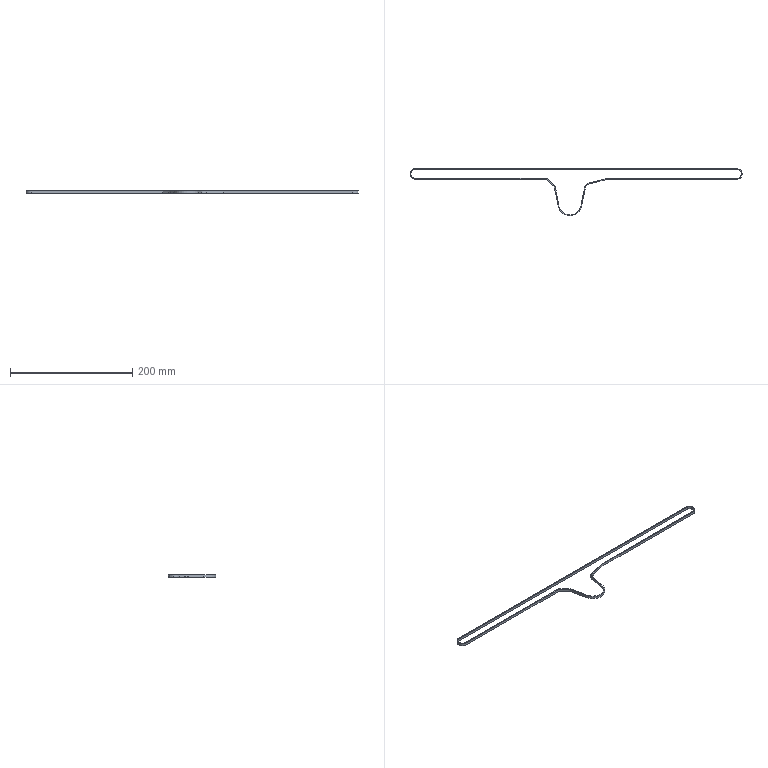Part | STEP file | Anti-static belt | 1 solid | 30 faces | box 544 x 77.5 x 4 mm | volume 7074 mm3 | plane 16 | cylinder 14 | commonest cylinder face diameters 18 x5 15 x3 37 x3 21 x2 40 x1